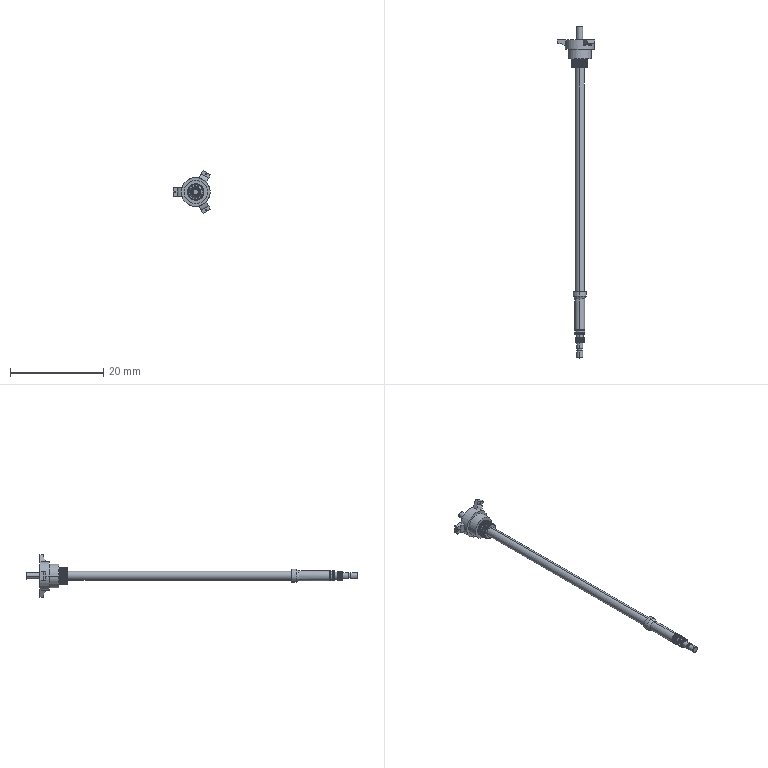Part | SolidWorks | features ICE 5, CirPattern 4, Fillet 3, Cut 2, Revolution 2 | 1 solid | 637 faces | box 7.952 x 71.26 x 9.182 mm | volume 329.036 mm3 | plane 502 | cylinder 125 | torus 8 | cone 2 | commonest cylinder face diameters 2.013 x48 3.5 x48 0.237 x6 1.34 x4 4.501 x3 1.144 x2